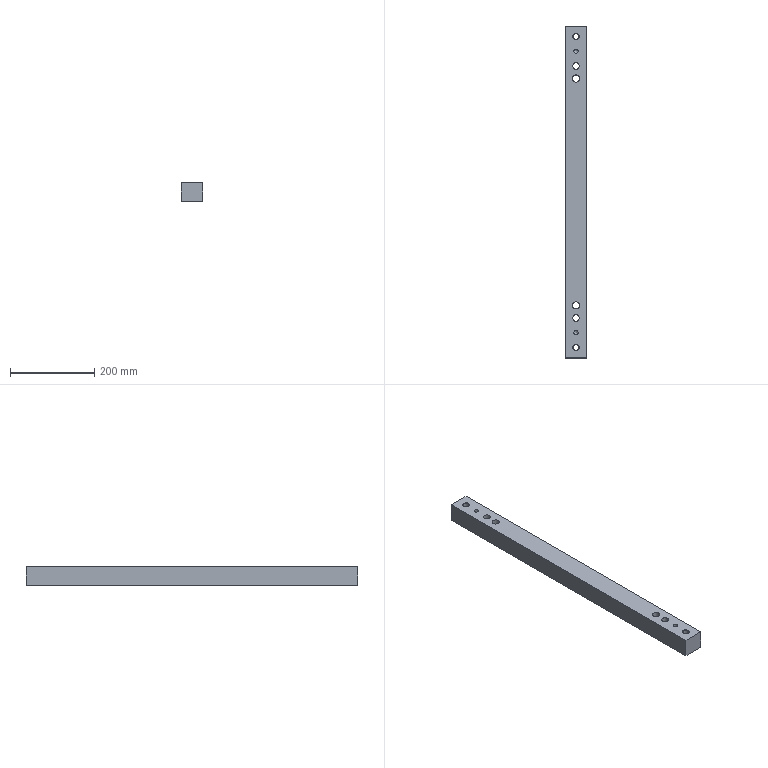Part | STEP file | 011_id2222_x_t | 1 solid | 18 faces | box 50 x 790 x 45 mm | volume 1720407 mm3 | cylinder 8 | plane 6 | cone 4 | commonest cylinder face diameters 10.3 x2 14 x2 16 x2 17 x2
STEP:
#1=CARTESIAN_POINT('',(0.,0.,0.));
#2=DIRECTION('',(0.,0.,1.));
#3=DIRECTION('',(1.,0.,0.));
#4=AXIS2_PLACEMENT_3D('',#1,#2,#3);
#5=CARTESIAN_POINT('',(-933.5,370.,185.));
#6=VERTEX_POINT('',#5);
#7=CARTESIAN_POINT('',(-919.5,370.,185.));
#8=VERTEX_POINT('',#7);
#9=CARTESIAN_POINT('',(-926.5,370.,185.));
#10=DIRECTION('',(0.,0.,-1.));
#11=DIRECTION('',(-1.,0.,0.));
#12=AXIS2_PLACEMENT_3D('',#9,#10,#11);
#13=CIRCLE('',#12,7.);
#14=CARTESIAN_POINT('',(173.5,0.,185.));
#15=DIRECTION('',(0.,0.,-1.));
#16=DIRECTION('',(1.,0.,0.));
#17=AXIS2_PLACEMENT_3D('',#14,#15,#16);
#18=PLANE('',#17);
#19=CARTESIAN_POINT('',(-1100.,-370.));
#20=DIRECTION('',(-1.,0.));
#21=AXIS2_PLACEMENT_2D('',#19,#20);
#22=CIRCLE('',#21,7.);
#23=(GEOMETRIC_REPRESENTATION_CONTEXT(2)PARAMETRIC_REPRESENTATION_CONTEXT()REPRESENTATION_CONTEXT('',''));
#24=DEFINITIONAL_REPRESENTATION('',(#22),#23);
#25=PCURVE('',#18,#24);
#26=CARTESIAN_POINT('',(-926.5,370.,230.));
#27=DIRECTION('',(0.,0.,-1.));
#28=DIRECTION('',(1.,0.,0.));
#29=AXIS2_PLACEMENT_3D('',#26,#27,#28);
#30=CYLINDRICAL_SURFACE('',#29,7.);
#31=CARTESIAN_POINT('',(3.142,45.));
#32=DIRECTION('',(1.,0.));
#33=VECTOR('',#32,1.);
#34=LINE('',#31,#33);
#35=(GEOMETRIC_REPRESENTATION_CONTEXT(2)PARAMETRIC_REPRESENTATION_CONTEXT()REPRESENTATION_CONTEXT('',''));
#36=DEFINITIONAL_REPRESENTATION('',(#34),#35);
#37=PCURVE('',#30,#36);
#38=SURFACE_CURVE('',#13,(#25,#37),.PCURVE_S1.);
#39=EDGE_CURVE('',#6,#8,#38,.T.);
#40=ORIENTED_EDGE('',*,*,#39,.F.);
#41=CARTESIAN_POINT('',(-926.5,370.,185.));
#42=DIRECTION('',(0.,0.,-1.));
#43=DIRECTION('',(-1.,0.,0.));
#44=AXIS2_PLACEMENT_3D('',#41,#42,#43);
#45=CIRCLE('',#44,7.);
#46=CARTESIAN_POINT('',(-1100.,-370.));
#47=DIRECTION('',(-1.,0.));
#48=AXIS2_PLACEMENT_2D('',#46,#47);
#49=CIRCLE('',#48,7.);
#50=(GEOMETRIC_REPRESENTATION_CONTEXT(2)PARAMETRIC_REPRESENTATION_CONTEXT()REPRESENTATION_CONTEXT('',''));
#51=DEFINITIONAL_REPRESENTATION('',(#49),#50);
#52=PCURVE('',#18,#51);
#53=CARTESIAN_POINT('',(-3.142,45.));
#54=DIRECTION('',(1.,0.));
#55=VECTOR('',#54,1.);
#56=LINE('',#53,#55);
#57=(GEOMETRIC_REPRESENTATION_CONTEXT(2)PARAMETRIC_REPRESENTATION_CONTEXT()REPRESENTATION_CONTEXT('',''));
#58=DEFINITIONAL_REPRESENTATION('',(#56),#57);
#59=PCURVE('',#30,#58);
#60=SURFACE_CURVE('',#45,(#52,#59),.PCURVE_S1.);
#61=EDGE_CURVE('',#8,#6,#60,.T.);
#62=ORIENTED_EDGE('',*,*,#61,.F.);
#63=EDGE_LOOP('',(#40,#62));
#64=FACE_BOUND('',#63,.T.);
#65=CARTESIAN_POINT('',(-934.5,-300.,185.));
#66=VERTEX_POINT('',#65);
#67=CARTESIAN_POINT('',(-918.5,-300.,185.));
#68=VERTEX_POINT('',#67);
#69=CARTESIAN_POINT('',(-926.5,-300.,185.));
#70=DIRECTION('',(0.,0.,-1.));
#71=DIRECTION('',(-1.,0.,0.));
#72=AXIS2_PLACEMENT_3D('',#69,#70,#71);
#73=CIRCLE('',#72,8.);
#74=CARTESIAN_POINT('',(-1100.,300.));
#75=DIRECTION('',(-1.,0.));
#76=AXIS2_PLACEMENT_2D('',#74,#75);
#77=CIRCLE('',#76,8.);
#78=(GEOMETRIC_REPRESENTATION_CONTEXT(2)PARAMETRIC_REPRESENTATION_CONTEXT()REPRESENTATION_CONTEXT('',''));
#79=DEFINITIONAL_REPRESENTATION('',(#77),#78);
#80=PCURVE('',#18,#79);
#81=CARTESIAN_POINT('',(-926.5,-300.,310.));
#82=DIRECTION('',(0.,0.,-1.));
#83=DIRECTION('',(1.,0.,0.));
#84=AXIS2_PLACEMENT_3D('',#81,#82,#83);
#85=CYLINDRICAL_SURFACE('',#84,8.);
#86=CARTESIAN_POINT('',(3.142,125.));
#87=DIRECTION('',(1.,0.));
#88=VECTOR('',#87,1.);
#89=LINE('',#86,#88);
#90=(GEOMETRIC_REPRESENTATION_CONTEXT(2)PARAMETRIC_REPRESENTATION_CONTEXT()REPRESENTATION_CONTEXT('',''));
#91=DEFINITIONAL_REPRESENTATION('',(#89),#90);
#92=PCURVE('',#85,#91);
#93=SURFACE_CURVE('',#73,(#80,#92),.PCURVE_S1.);
#94=EDGE_CURVE('',#66,#68,#93,.T.);
#95=ORIENTED_EDGE('',*,*,#94,.F.);
#96=CARTESIAN_POINT('',(-926.5,-300.,185.));
#97=DIRECTION('',(0.,0.,-1.));
#98=DIRECTION('',(-1.,0.,0.));
#99=AXIS2_PLACEMENT_3D('',#96,#97,#98);
#100=CIRCLE('',#99,8.);
#101=CARTESIAN_POINT('',(-1100.,300.));
#102=DIRECTION('',(-1.,0.));
#103=AXIS2_PLACEMENT_2D('',#101,#102);
#104=CIRCLE('',#103,8.);
#105=(GEOMETRIC_REPRESENTATION_CONTEXT(2)PARAMETRIC_REPRESENTATION_CONTEXT()REPRESENTATION_CONTEXT('',''));
#106=DEFINITIONAL_REPRESENTATION('',(#104),#105);
#107=PCURVE('',#18,#106);
#108=CARTESIAN_POINT('',(-3.142,125.));
#109=DIRECTION('',(1.,0.));
#110=VECTOR('',#109,1.);
#111=LINE('',#108,#110);
#112=(GEOMETRIC_REPRESENTATION_CONTEXT(2)PARAMETRIC_REPRESENTATION_CONTEXT()REPRESENTATION_CONTEXT('',''));
#113=DEFINITIONAL_REPRESENTATION('',(#111),#112);
#114=PCURVE('',#85,#113);
#115=SURFACE_CURVE('',#100,(#107,#114),.PCURVE_S1.);
#116=EDGE_CURVE('',#68,#66,#115,.T.);
#117=ORIENTED_EDGE('',*,*,#116,.F.);
#118=EDGE_LOOP('',(#95,#117));
#119=FACE_BOUND('',#118,.T.);
#120=CARTESIAN_POINT('',(-934.5,300.,185.));
#121=VERTEX_POINT('',#120);
#122=CARTESIAN_POINT('',(-918.5,300.,185.));
#123=VERTEX_POINT('',#122);
#124=CARTESIAN_POINT('',(-926.5,300.,185.));
#125=DIRECTION('',(0.,0.,-1.));
#126=DIRECTION('',(-1.,0.,0.));
#127=AXIS2_PLACEMENT_3D('',#124,#125,#126);
#128=CIRCLE('',#127,8.);
#129=CARTESIAN_POINT('',(-1100.,-300.));
#130=DIRECTION('',(-1.,0.));
#131=AXIS2_PLACEMENT_2D('',#129,#130);
#132=CIRCLE('',#131,8.);
#133=(GEOMETRIC_REPRESENTATION_CONTEXT(2)PARAMETRIC_REPRESENTATION_CONTEXT()REPRESENTATION_CONTEXT('',''));
#134=DEFINITIONAL_REPRESENTATION('',(#132),#133);
#135=PCURVE('',#18,#134);
#136=CARTESIAN_POINT('',(-926.5,300.,310.));
#137=DIRECTION('',(0.,0.,-1.));
#138=DIRECTION('',(1.,0.,0.));
#139=AXIS2_PLACEMENT_3D('',#136,#137,#138);
#140=CYLINDRICAL_SURFACE('',#139,8.);
#141=CARTESIAN_POINT('',(3.142,125.));
#142=DIRECTION('',(1.,0.));
#143=VECTOR('',#142,1.);
#144=LINE('',#141,#143);
#145=(GEOMETRIC_REPRESENTATION_CONTEXT(2)PARAMETRIC_REPRESENTATION_CONTEXT()REPRESENTATION_CONTEXT('',''));
#146=DEFINITIONAL_REPRESENTATION('',(#144),#145);
#147=PCURVE('',#140,#146);
#148=SURFACE_CURVE('',#128,(#135,#147),.PCURVE_S1.);
#149=EDGE_CURVE('',#121,#123,#148,.T.);
#150=ORIENTED_EDGE('',*,*,#149,.F.);
#151=CARTESIAN_POINT('',(-926.5,300.,185.));
#152=DIRECTION('',(0.,0.,-1.));
#153=DIRECTION('',(-1.,0.,0.));
#154=AXIS2_PLACEMENT_3D('',#151,#152,#153);
#155=CIRCLE('',#154,8.);
#156=CARTESIAN_POINT('',(-1100.,-300.));
#157=DIRECTION('',(-1.,0.));
#158=AXIS2_PLACEMENT_2D('',#156,#157);
#159=CIRCLE('',#158,8.);
#160=(GEOMETRIC_REPRESENTATION_CONTEXT(2)PARAMETRIC_REPRESENTATION_CONTEXT()REPRESENTATION_CONTEXT('',''));
#161=DEFINITIONAL_REPRESENTATION('',(#159),#160);
#162=PCURVE('',#18,#161);
#163=CARTESIAN_POINT('',(-3.142,125.));
#164=DIRECTION('',(1.,0.));
#165=VECTOR('',#164,1.);
#166=LINE('',#163,#165);
#167=(GEOMETRIC_REPRESENTATION_CONTEXT(2)PARAMETRIC_REPRESENTATION_CONTEXT()REPRESENTATION_CONTEXT('',''));
#168=DEFINITIONAL_REPRESENTATION('',(#166),#167);
#169=PCURVE('',#140,#168);
#170=SURFACE_CURVE('',#155,(#162,#169),.PCURVE_S1.);
#171=EDGE_CURVE('',#123,#121,#170,.T.);
#172=ORIENTED_EDGE('',*,*,#171,.F.);
#173=EDGE_LOOP('',(#150,#172));
#174=FACE_BOUND('',#173,.T.);
#175=CARTESIAN_POINT('',(-951.5,-395.,185.));
#176=VERTEX_POINT('',#175);
#177=CARTESIAN_POINT('',(-951.5,395.,185.));
#178=VERTEX_POINT('',#177);
#179=CARTESIAN_POINT('',(-951.5,0.,185.));
#180=DIRECTION('',(0.,1.,0.));
#181=VECTOR('',#180,1.);
#182=LINE('',#179,#181);
#183=CARTESIAN_POINT('',(-1125.,0.));
#184=DIRECTION('',(0.,-1.));
#185=VECTOR('',#184,1.);
#186=LINE('',#183,#185);
#187=(GEOMETRIC_REPRESENTATION_CONTEXT(2)PARAMETRIC_REPRESENTATION_CONTEXT()REPRESENTATION_CONTEXT('',''));
#188=DEFINITIONAL_REPRESENTATION('',(#186),#187);
#189=PCURVE('',#18,#188);
#190=CARTESIAN_POINT('',(-951.5,-210.,-28.5));
#191=DIRECTION('',(-1.,0.,0.));
#192=DIRECTION('',(0.,0.,1.));
#193=AXIS2_PLACEMENT_3D('',#190,#191,#192);
#194=PLANE('',#193);
#195=CARTESIAN_POINT('',(213.5,210.));
#196=DIRECTION('',(0.,1.));
#197=VECTOR('',#196,1.);
#198=LINE('',#195,#197);
#199=(GEOMETRIC_REPRESENTATION_CONTEXT(2)PARAMETRIC_REPRESENTATION_CONTEXT()REPRESENTATION_CONTEXT('',''));
#200=DEFINITIONAL_REPRESENTATION('',(#198),#199);
#201=PCURVE('',#194,#200);
#202=SURFACE_CURVE('',#182,(#189,#201),.PCURVE_S1.);
#203=EDGE_CURVE('',#176,#178,#202,.T.);
#204=ORIENTED_EDGE('',*,*,#203,.T.);
#205=CARTESIAN_POINT('',(-901.5,395.,185.));
#206=VERTEX_POINT('',#205);
#207=CARTESIAN_POINT('',(-951.5,395.,185.));
#208=DIRECTION('',(-1.,0.,0.));
#209=VECTOR('',#208,1.);
#210=LINE('',#207,#209);
#211=CARTESIAN_POINT('',(-1125.,-395.));
#212=DIRECTION('',(-1.,0.));
#213=VECTOR('',#212,1.);
#214=LINE('',#211,#213);
#215=(GEOMETRIC_REPRESENTATION_CONTEXT(2)PARAMETRIC_REPRESENTATION_CONTEXT()REPRESENTATION_CONTEXT('',''));
#216=DEFINITIONAL_REPRESENTATION('',(#214),#215);
#217=PCURVE('',#18,#216);
#218=CARTESIAN_POINT('',(-951.5,395.,-28.5));
#219=DIRECTION('',(0.,1.,0.));
#220=DIRECTION('',(0.,0.,-1.));
#221=AXIS2_PLACEMENT_3D('',#218,#219,#220);
#222=PLANE('',#221);
#223=CARTESIAN_POINT('',(-213.5,0.));
#224=DIRECTION('',(0.,1.));
#225=VECTOR('',#224,1.);
#226=LINE('',#223,#225);
#227=(GEOMETRIC_REPRESENTATION_CONTEXT(2)PARAMETRIC_REPRESENTATION_CONTEXT()REPRESENTATION_CONTEXT('',''));
#228=DEFINITIONAL_REPRESENTATION('',(#226),#227);
#229=PCURVE('',#222,#228);
#230=SURFACE_CURVE('',#210,(#217,#229),.PCURVE_S1.);
#231=EDGE_CURVE('',#206,#178,#230,.T.);
#232=ORIENTED_EDGE('',*,*,#231,.F.);
#233=CARTESIAN_POINT('',(-901.5,-395.,185.));
#234=VERTEX_POINT('',#233);
#235=CARTESIAN_POINT('',(-901.5,-210.,185.));
#236=DIRECTION('',(0.,-1.,0.));
#237=VECTOR('',#236,1.);
#238=LINE('',#235,#237);
#239=CARTESIAN_POINT('',(-1075.,210.));
#240=DIRECTION('',(0.,1.));
#241=VECTOR('',#240,1.);
#242=LINE('',#239,#241);
#243=(GEOMETRIC_REPRESENTATION_CONTEXT(2)PARAMETRIC_REPRESENTATION_CONTEXT()REPRESENTATION_CONTEXT('',''));
#244=DEFINITIONAL_REPRESENTATION('',(#242),#243);
#245=PCURVE('',#18,#244);
#246=CARTESIAN_POINT('',(-901.5,-210.,-28.5));
#247=DIRECTION('',(-1.,0.,0.));
#248=DIRECTION('',(0.,0.,1.));
#249=AXIS2_PLACEMENT_3D('',#246,#247,#248);
#250=PLANE('',#249);
#251=CARTESIAN_POINT('',(213.5,0.));
#252=DIRECTION('',(0.,-1.));
#253=VECTOR('',#252,1.);
#254=LINE('',#251,#253);
#255=(GEOMETRIC_REPRESENTATION_CONTEXT(2)PARAMETRIC_REPRESENTATION_CONTEXT()REPRESENTATION_CONTEXT('',''));
#256=DEFINITIONAL_REPRESENTATION('',(#254),#255);
#257=PCURVE('',#250,#256);
#258=SURFACE_CURVE('',#238,(#245,#257),.PCURVE_S1.);
#259=EDGE_CURVE('',#206,#234,#258,.T.);
#260=ORIENTED_EDGE('',*,*,#259,.T.);
#261=CARTESIAN_POINT('',(173.5,-395.,185.));
#262=DIRECTION('',(1.,0.,0.));
#263=VECTOR('',#262,1.);
#264=LINE('',#261,#263);
#265=CARTESIAN_POINT('',(0.,395.));
#266=DIRECTION('',(1.,0.));
#267=VECTOR('',#266,1.);
#268=LINE('',#265,#267);
#269=(GEOMETRIC_REPRESENTATION_CONTEXT(2)PARAMETRIC_REPRESENTATION_CONTEXT()REPRESENTATION_CONTEXT('',''));
#270=DEFINITIONAL_REPRESENTATION('',(#268),#269);
#271=PCURVE('',#18,#270);
#272=CARTESIAN_POINT('',(-951.5,-395.,-28.5));
#273=DIRECTION('',(0.,1.,0.));
#274=DIRECTION('',(0.,0.,-1.));
#275=AXIS2_PLACEMENT_3D('',#272,#273,#274);
#276=PLANE('',#275);
#277=CARTESIAN_POINT('',(-213.5,-1125.));
#278=DIRECTION('',(0.,-1.));
#279=VECTOR('',#278,1.);
#280=LINE('',#277,#279);
#281=(GEOMETRIC_REPRESENTATION_CONTEXT(2)PARAMETRIC_REPRESENTATION_CONTEXT()REPRESENTATION_CONTEXT('',''));
#282=DEFINITIONAL_REPRESENTATION('',(#280),#281);
#283=PCURVE('',#276,#282);
#284=SURFACE_CURVE('',#264,(#271,#283),.PCURVE_S1.);
#285=EDGE_CURVE('',#176,#234,#284,.T.);
#286=ORIENTED_EDGE('',*,*,#285,.F.);
#287=EDGE_LOOP('',(#204,#232,#260,#286));
#288=FACE_BOUND('',#287,.T.);
#289=CARTESIAN_POINT('',(-933.5,-370.,185.));
#290=VERTEX_POINT('',#289);
#291=CARTESIAN_POINT('',(-919.5,-370.,185.));
#292=VERTEX_POINT('',#291);
#293=CARTESIAN_POINT('',(-926.5,-370.,185.));
#294=DIRECTION('',(0.,0.,-1.));
#295=DIRECTION('',(-1.,0.,0.));
#296=AXIS2_PLACEMENT_3D('',#293,#294,#295);
#297=CIRCLE('',#296,7.);
#298=CARTESIAN_POINT('',(-1100.,370.));
#299=DIRECTION('',(-1.,0.));
#300=AXIS2_PLACEMENT_2D('',#298,#299);
#301=CIRCLE('',#300,7.);
#302=(GEOMETRIC_REPRESENTATION_CONTEXT(2)PARAMETRIC_REPRESENTATION_CONTEXT()REPRESENTATION_CONTEXT('',''));
#303=DEFINITIONAL_REPRESENTATION('',(#301),#302);
#304=PCURVE('',#18,#303);
#305=CARTESIAN_POINT('',(-926.5,-370.,230.));
#306=DIRECTION('',(0.,0.,-1.));
#307=DIRECTION('',(1.,0.,0.));
#308=AXIS2_PLACEMENT_3D('',#305,#306,#307);
#309=CYLINDRICAL_SURFACE('',#308,7.);
#310=CARTESIAN_POINT('',(3.142,45.));
#311=DIRECTION('',(1.,0.));
#312=VECTOR('',#311,1.);
#313=LINE('',#310,#312);
#314=(GEOMETRIC_REPRESENTATION_CONTEXT(2)PARAMETRIC_REPRESENTATION_CONTEXT()REPRESENTATION_CONTEXT('',''));
#315=DEFINITIONAL_REPRESENTATION('',(#313),#314);
#316=PCURVE('',#309,#315);
#317=SURFACE_CURVE('',#297,(#304,#316),.PCURVE_S1.);
#318=EDGE_CURVE('',#290,#292,#317,.T.);
#319=ORIENTED_EDGE('',*,*,#318,.F.);
#320=CARTESIAN_POINT('',(-926.5,-370.,185.));
#321=DIRECTION('',(0.,0.,-1.));
#322=DIRECTION('',(-1.,0.,0.));
#323=AXIS2_PLACEMENT_3D('',#320,#321,#322);
#324=CIRCLE('',#323,7.);
#325=CARTESIAN_POINT('',(-1100.,370.));
#326=DIRECTION('',(-1.,0.));
#327=AXIS2_PLACEMENT_2D('',#325,#326);
#328=CIRCLE('',#327,7.);
#329=(GEOMETRIC_REPRESENTATION_CONTEXT(2)PARAMETRIC_REPRESENTATION_CONTEXT()REPRESENTATION_CONTEXT('',''));
#330=DEFINITIONAL_REPRESENTATION('',(#328),#329);
#331=PCURVE('',#18,#330);
#332=CARTESIAN_POINT('',(-3.142,45.));
#333=DIRECTION('',(1.,0.));
#334=VECTOR('',#333,1.);
#335=LINE('',#332,#334);
#336=(GEOMETRIC_REPRESENTATION_CONTEXT(2)PARAMETRIC_REPRESENTATION_CONTEXT()REPRESENTATION_CONTEXT('',''));
#337=DEFINITIONAL_REPRESENTATION('',(#335),#336);
#338=PCURVE('',#309,#337);
#339=SURFACE_CURVE('',#324,(#331,#338),.PCURVE_S1.);
#340=EDGE_CURVE('',#292,#290,#339,.T.);
#341=ORIENTED_EDGE('',*,*,#340,.F.);
#342=EDGE_LOOP('',(#319,#341));
#343=FACE_BOUND('',#342,.T.);
#344=CARTESIAN_POINT('',(-935.,-270.,185.));
#345=VERTEX_POINT('',#344);
#346=CARTESIAN_POINT('',(-926.5,-270.,185.));
#347=DIRECTION('',(0.,0.,-1.));
#348=DIRECTION('',(-1.,0.,0.));
#349=AXIS2_PLACEMENT_3D('',#346,#347,#348);
#350=CIRCLE('',#349,8.5);
#351=CARTESIAN_POINT('',(-1100.,270.));
#352=DIRECTION('',(-1.,0.));
#353=AXIS2_PLACEMENT_2D('',#351,#352);
#354=CIRCLE('',#353,8.5);
#355=(GEOMETRIC_REPRESENTATION_CONTEXT(2)PARAMETRIC_REPRESENTATION_CONTEXT()REPRESENTATION_CONTEXT('',''));
#356=DEFINITIONAL_REPRESENTATION('',(#354),#355);
#357=PCURVE('',#18,#356);
#358=CARTESIAN_POINT('',(-926.5,-270.,150.));
#359=DIRECTION('',(0.,0.,1.));
#360=DIRECTION('',(1.,0.,0.));
#361=AXIS2_PLACEMENT_3D('',#358,#359,#360);
#362=CYLINDRICAL_SURFACE('',#361,8.5);
#363=CARTESIAN_POINT('',(9.425,35.));
#364=DIRECTION('',(-1.,0.));
#365=VECTOR('',#364,1.);
#366=LINE('',#363,#365);
#367=(GEOMETRIC_REPRESENTATION_CONTEXT(2)PARAMETRIC_REPRESENTATION_CONTEXT()REPRESENTATION_CONTEXT('',''));
#368=DEFINITIONAL_REPRESENTATION('',(#366),#367);
#369=PCURVE('',#362,#368);
#370=SURFACE_CURVE('',#350,(#357,#369),.PCURVE_S1.);
#371=EDGE_CURVE('',#345,#345,#370,.T.);
#372=ORIENTED_EDGE('',*,*,#371,.F.);
#373=EDGE_LOOP('',(#372));
#374=FACE_BOUND('',#373,.T.);
#375=CARTESIAN_POINT('',(-935.,270.,185.));
#376=VERTEX_POINT('',#375);
#377=CARTESIAN_POINT('',(-926.5,270.,185.));
#378=DIRECTION('',(0.,0.,1.));
#379=DIRECTION('',(-1.,0.,0.));
#380=AXIS2_PLACEMENT_3D('',#377,#378,#379);
#381=CIRCLE('',#380,8.5);
#382=CARTESIAN_POINT('',(-1108.5,-270.));
#383=CARTESIAN_POINT('',(-1108.5,-255.278));
#384=CARTESIAN_POINT('',(-1095.75,-262.639));
#385=CARTESIAN_POINT('',(-1083.,-270.));
#386=CARTESIAN_POINT('',(-1095.75,-277.361));
#387=CARTESIAN_POINT('',(-1108.5,-284.722));
#388=CARTESIAN_POINT('',(-1108.5,-270.));
#389=(BOUNDED_CURVE()B_SPLINE_CURVE(2,(#382,#383,#384,#385,#386,#387,#388),.UNSPECIFIED.,.T.,.F.)B_SPLINE_CURVE_WITH_KNOTS((1,2,2,2,2,1),(-2.094,0.,2.094,4.189,6.283,8.378),.UNSPECIFIED.)CURVE()GEOMETRIC_REPRESENTATION_ITEM()RATIONAL_B_SPLINE_CURVE((1.,0.5,1.,0.5,1.,0.5,1.))REPRESENTATION_ITEM(''));
#390=(GEOMETRIC_REPRESENTATION_CONTEXT(2)PARAMETRIC_REPRESENTATION_CONTEXT()REPRESENTATION_CONTEXT('',''));
#391=DEFINITIONAL_REPRESENTATION('',(#389),#390);
#392=PCURVE('',#18,#391);
#393=CARTESIAN_POINT('',(-926.5,270.,150.));
#394=DIRECTION('',(0.,0.,1.));
#395=DIRECTION('',(1.,0.,0.));
#396=AXIS2_PLACEMENT_3D('',#393,#394,#395);
#397=CYLINDRICAL_SURFACE('',#396,8.5);
#398=CARTESIAN_POINT('',(3.142,35.));
#399=DIRECTION('',(1.,0.));
#400=VECTOR('',#399,1.);
#401=LINE('',#398,#400);
#402=(GEOMETRIC_REPRESENTATION_CONTEXT(2)PARAMETRIC_REPRESENTATION_CONTEXT()REPRESENTATION_CONTEXT('',''));
#403=DEFINITIONAL_REPRESENTATION('',(#401),#402);
#404=PCURVE('',#397,#403);
#405=SURFACE_CURVE('',#381,(#392,#404),.PCURVE_S1.);
#406=EDGE_CURVE('',#376,#376,#405,.T.);
#407=ORIENTED_EDGE('',*,*,#406,.T.);
#408=EDGE_LOOP('',(#407));
#409=FACE_BOUND('',#408,.T.);
#410=ADVANCED_FACE('',(#64,#119,#174,#288,#343,#374,#409),#18,.T.);
#411=CARTESIAN_POINT('',(-931.65,-335.,230.));
#412=VERTEX_POINT('',#411);
#413=CARTESIAN_POINT('',(-926.5,-335.,230.));
#414=DIRECTION('',(0.,0.,-1.));
#415=DIRECTION('',(-1.,0.,0.));
#416=AXIS2_PLACEMENT_3D('',#413,#414,#415);
#417=CIRCLE('',#416,5.15);
#418=CARTESIAN_POINT('',(-951.5,-210.,230.));
#419=DIRECTION('',(0.,0.,-1.));
#420=DIRECTION('',(0.,-1.,0.));
#421=AXIS2_PLACEMENT_3D('',#418,#419,#420);
#422=PLANE('',#421);
#423=CARTESIAN_POINT('',(125.,-25.));
#424=DIRECTION('',(0.,1.));
#425=AXIS2_PLACEMENT_2D('',#423,#424);
#426=CIRCLE('',#425,5.15);
#427=(GEOMETRIC_REPRESENTATION_CONTEXT(2)PARAMETRIC_REPRESENTATION_CONTEXT()REPRESENTATION_CONTEXT('',''));
#428=DEFINITIONAL_REPRESENTATION('',(#426),#427);
#429=PCURVE('',#422,#428);
#430=CARTESIAN_POINT('',(-926.5,-335.,259.));
#431=DIRECTION('',(0.,0.,-1.));
#432=DIRECTION('',(-1.,0.,0.));
#433=AXIS2_PLACEMENT_3D('',#430,#431,#432);
#434=CYLINDRICAL_SURFACE('',#433,5.15);
#435=CARTESIAN_POINT('',(0.,29.));
#436=DIRECTION('',(1.,0.));
#437=VECTOR('',#436,1.);
#438=LINE('',#435,#437);
#439=(GEOMETRIC_REPRESENTATION_CONTEXT(2)PARAMETRIC_REPRESENTATION_CONTEXT()REPRESENTATION_CONTEXT('',''));
#440=DEFINITIONAL_REPRESENTATION('',(#438),#439);
#441=PCURVE('',#434,#440);
#442=SURFACE_CURVE('',#417,(#429,#441),.PCURVE_S1.);
#443=EDGE_CURVE('',#412,#412,#442,.T.);
#444=ORIENTED_EDGE('',*,*,#443,.T.);
#445=EDGE_LOOP('',(#444));
#446=FACE_BOUND('',#445,.T.);
#447=CARTESIAN_POINT('',(-931.65,335.,230.));
#448=VERTEX_POINT('',#447);
#449=CARTESIAN_POINT('',(-926.5,335.,230.));
#450=DIRECTION('',(0.,0.,1.));
#451=DIRECTION('',(-1.,0.,0.));
#452=AXIS2_PLACEMENT_3D('',#449,#450,#451);
#453=CIRCLE('',#452,5.15);
#454=CARTESIAN_POINT('',(-545.,-19.85));
#455=CARTESIAN_POINT('',(-536.08,-19.85));
#456=CARTESIAN_POINT('',(-540.54,-27.575));
#457=CARTESIAN_POINT('',(-545.,-35.3));
#458=CARTESIAN_POINT('',(-549.46,-27.575));
#459=CARTESIAN_POINT('',(-553.92,-19.85));
#460=CARTESIAN_POINT('',(-545.,-19.85));
#461=(BOUNDED_CURVE()B_SPLINE_CURVE(2,(#454,#455,#456,#457,#458,#459,#460),.UNSPECIFIED.,.T.,.F.)B_SPLINE_CURVE_WITH_KNOTS((1,2,2,2,2,1),(-2.094,0.,2.094,4.189,6.283,8.378),.UNSPECIFIED.)CURVE()GEOMETRIC_REPRESENTATION_ITEM()RATIONAL_B_SPLINE_CURVE((1.,0.5,1.,0.5,1.,0.5,1.))REPRESENTATION_ITEM(''));
#462=(GEOMETRIC_REPRESENTATION_CONTEXT(2)PARAMETRIC_REPRESENTATION_CONTEXT()REPRESENTATION_CONTEXT('',''));
#463=DEFINITIONAL_REPRESENTATION('',(#461),#462);
#464=PCURVE('',#422,#463);
#465=CARTESIAN_POINT('',(-926.5,335.,259.));
#466=DIRECTION('',(0.,0.,-1.));
#467=DIRECTION('',(-1.,0.,0.));
#468=AXIS2_PLACEMENT_3D('',#465,#466,#467);
#469=CYLINDRICAL_SURFACE('',#468,5.15);
#470=CARTESIAN_POINT('',(6.283,29.));
#471=DIRECTION('',(-1.,0.));
#472=VECTOR('',#471,1.);
#473=LINE('',#470,#472);
#474=(GEOMETRIC_REPRESENTATION_CONTEXT(2)PARAMETRIC_REPRESENTATION_CONTEXT()REPRESENTATION_CONTEXT('',''));
#475=DEFINITIONAL_REPRESENTATION('',(#473),#474);
#476=PCURVE('',#469,#475);
#477=SURFACE_CURVE('',#453,(#464,#476),.PCURVE_S1.);
#478=EDGE_CURVE('',#448,#448,#477,.T.);
#479=ORIENTED_EDGE('',*,*,#478,.F.);
#480=EDGE_LOOP('',(#479));
#481=FACE_BOUND('',#480,.T.);
#482=CARTESIAN_POINT('',(-935.,270.,230.));
#483=VERTEX_POINT('',#482);
#484=CARTESIAN_POINT('',(-926.5,270.,230.));
#485=DIRECTION('',(0.,0.,1.));
#486=DIRECTION('',(-1.,0.,0.));
#487=AXIS2_PLACEMENT_3D('',#484,#485,#486);
#488=CIRCLE('',#487,8.5);
#489=CARTESIAN_POINT('',(-480.,-16.5));
#490=CARTESIAN_POINT('',(-465.278,-16.5));
#491=CARTESIAN_POINT('',(-472.639,-29.25));
#492=CARTESIAN_POINT('',(-480.,-42.));
#493=CARTESIAN_POINT('',(-487.361,-29.25));
#494=CARTESIAN_POINT('',(-494.722,-16.5));
#495=CARTESIAN_POINT('',(-480.,-16.5));
#496=(BOUNDED_CURVE()B_SPLINE_CURVE(2,(#489,#490,#491,#492,#493,#494,#495),.UNSPECIFIED.,.T.,.F.)B_SPLINE_CURVE_WITH_KNOTS((1,2,2,2,2,1),(-2.094,0.,2.094,4.189,6.283,8.378),.UNSPECIFIED.)CURVE()GEOMETRIC_REPRESENTATION_ITEM()RATIONAL_B_SPLINE_CURVE((1.,0.5,1.,0.5,1.,0.5,1.))REPRESENTATION_ITEM(''));
#497=(GEOMETRIC_REPRESENTATION_CONTEXT(2)PARAMETRIC_REPRESENTATION_CONTEXT()REPRESENTATION_CONTEXT('',''));
#498=DEFINITIONAL_REPRESENTATION('',(#496),#497);
#499=PCURVE('',#422,#498);
#500=CARTESIAN_POINT('',(3.142,80.));
#501=DIRECTION('',(1.,0.));
#502=VECTOR('',#501,1.);
#503=LINE('',#500,#502);
#504=(GEOMETRIC_REPRESENTATION_CONTEXT(2)PARAMETRIC_REPRESENTATION_CONTEXT()REPRESENTATION_CONTEXT('',''));
#505=DEFINITIONAL_REPRESENTATION('',(#503),#504);
#506=PCURVE('',#397,#505);
#507=SURFACE_CURVE('',#488,(#499,#506),.PCURVE_S1.);
#508=EDGE_CURVE('',#483,#483,#507,.T.);
#509=ORIENTED_EDGE('',*,*,#508,.F.);
#510=EDGE_LOOP('',(#509));
#511=FACE_BOUND('',#510,.T.);
#512=CARTESIAN_POINT('',(-935.,-270.,230.));
#513=VERTEX_POINT('',#512);
#514=CARTESIAN_POINT('',(-926.5,-270.,230.));
#515=DIRECTION('',(0.,0.,-1.));
#516=DIRECTION('',(-1.,0.,0.));
#517=AXIS2_PLACEMENT_3D('',#514,#515,#516);
#518=CIRCLE('',#517,8.5);
#519=CARTESIAN_POINT('',(60.,-25.));
#520=DIRECTION('',(0.,1.));
#521=AXIS2_PLACEMENT_2D('',#519,#520);
#522=CIRCLE('',#521,8.5);
#523=(GEOMETRIC_REPRESENTATION_CONTEXT(2)PARAMETRIC_REPRESENTATION_CONTEXT()REPRESENTATION_CONTEXT('',''));
#524=DEFINITIONAL_REPRESENTATION('',(#522),#523);
#525=PCURVE('',#422,#524);
#526=CARTESIAN_POINT('',(9.425,80.));
#527=DIRECTION('',(-1.,0.));
#528=VECTOR('',#527,1.);
#529=LINE('',#526,#528);
#530=(GEOMETRIC_REPRESENTATION_CONTEXT(2)PARAMETRIC_REPRESENTATION_CONTEXT()REPRESENTATION_CONTEXT('',''));
#531=DEFINITIONAL_REPRESENTATION('',(#529),#530);
#532=PCURVE('',#362,#531);
#533=SURFACE_CURVE('',#518,(#525,#532),.PCURVE_S1.);
#534=EDGE_CURVE('',#513,#513,#533,.T.);
#535=ORIENTED_EDGE('',*,*,#534,.T.);
#536=EDGE_LOOP('',(#535));
#537=FACE_BOUND('',#536,.T.);
#538=CARTESIAN_POINT('',(-918.5,300.,230.));
#539=VERTEX_POINT('',#538);
#540=CARTESIAN_POINT('',(-926.5,300.,230.));
#541=DIRECTION('',(0.,0.,-1.));
#542=DIRECTION('',(-1.,0.,0.));
#543=AXIS2_PLACEMENT_3D('',#540,#541,#542);
#544=CIRCLE('',#543,8.);
#545=CARTESIAN_POINT('',(-510.,-25.));
#546=DIRECTION('',(0.,1.));
#547=AXIS2_PLACEMENT_2D('',#545,#546);
#548=CIRCLE('',#547,8.);
#549=(GEOMETRIC_REPRESENTATION_CONTEXT(2)PARAMETRIC_REPRESENTATION_CONTEXT()REPRESENTATION_CONTEXT('',''));
#550=DEFINITIONAL_REPRESENTATION('',(#548),#549);
#551=PCURVE('',#422,#550);
#552=CARTESIAN_POINT('',(-3.142,80.));
#553=DIRECTION('',(1.,0.));
#554=VECTOR('',#553,1.);
#555=LINE('',#552,#554);
#556=(GEOMETRIC_REPRESENTATION_CONTEXT(2)PARAMETRIC_REPRESENTATION_CONTEXT()REPRESENTATION_CONTEXT('',''));
#557=DEFINITIONAL_REPRESENTATION('',(#555),#556);
#558=PCURVE('',#140,#557);
#559=SURFACE_CURVE('',#544,(#551,#558),.PCURVE_S1.);
#560=EDGE_CURVE('',#539,#539,#559,.T.);
#561=ORIENTED_EDGE('',*,*,#560,.T.);
#562=EDGE_LOOP('',(#561));
#563=FACE_BOUND('',#562,.T.);
#564=CARTESIAN_POINT('',(-918.5,370.,230.));
#565=VERTEX_POINT('',#564);
#566=CARTESIAN_POINT('',(-926.5,370.,230.));
#567=DIRECTION('',(0.,0.,1.));
#568=DIRECTION('',(1.,0.,0.));
#569=AXIS2_PLACEMENT_3D('',#566,#567,#568);
#570=CIRCLE('',#569,8.);
#571=CARTESIAN_POINT('',(-580.,-33.));
#572=CARTESIAN_POINT('',(-593.856,-33.));
#573=CARTESIAN_POINT('',(-586.928,-21.));
#574=CARTESIAN_POINT('',(-580.,-9.));
#575=CARTESIAN_POINT('',(-573.072,-21.));
#576=CARTESIAN_POINT('',(-566.144,-33.));
#577=CARTESIAN_POINT('',(-580.,-33.));
#578=(BOUNDED_CURVE()B_SPLINE_CURVE(2,(#571,#572,#573,#574,#575,#576,#577),.UNSPECIFIED.,.T.,.F.)B_SPLINE_CURVE_WITH_KNOTS((1,2,2,2,2,1),(-2.094,0.,2.094,4.189,6.283,8.378),.UNSPECIFIED.)CURVE()GEOMETRIC_REPRESENTATION_ITEM()RATIONAL_B_SPLINE_CURVE((1.,0.5,1.,0.5,1.,0.5,1.))REPRESENTATION_ITEM(''));
#579=(GEOMETRIC_REPRESENTATION_CONTEXT(2)PARAMETRIC_REPRESENTATION_CONTEXT()REPRESENTATION_CONTEXT('',''));
#580=DEFINITIONAL_REPRESENTATION('',(#578),#579);
#581=PCURVE('',#422,#580);
#582=CARTESIAN_POINT('',(-926.5,370.,230.));
#583=DIRECTION('',(0.,0.,1.));
#584=DIRECTION('',(-1.,0.,0.));
#585=AXIS2_PLACEMENT_3D('',#582,#583,#584);
#586=CONICAL_SURFACE('',#585,8.,0.7854);
#587=CARTESIAN_POINT('',(3.142,0.));
#588=DIRECTION('',(1.,0.));
#589=VECTOR('',#588,1.);
#590=LINE('',#587,#589);
#591=(GEOMETRIC_REPRESENTATION_CONTEXT(2)PARAMETRIC_REPRESENTATION_CONTEXT()REPRESENTATION_CONTEXT('',''));
#592=DEFINITIONAL_REPRESENTATION('',(#590),#591);
#593=PCURVE('',#586,#592);
#594=SURFACE_CURVE('',#570,(#581,#593),.PCURVE_S1.);
#595=EDGE_CURVE('',#565,#565,#594,.T.);
#596=ORIENTED_EDGE('',*,*,#595,.F.);
#597=EDGE_LOOP('',(#596));
#598=FACE_BOUND('',#597,.T.);
#599=CARTESIAN_POINT('',(-918.5,-370.,230.));
#600=VERTEX_POINT('',#599);
#601=CARTESIAN_POINT('',(-926.5,-370.,230.));
#602=DIRECTION('',(0.,0.,1.));
#603=DIRECTION('',(1.,0.,0.));
#604=AXIS2_PLACEMENT_3D('',#601,#602,#603);
#605=CIRCLE('',#604,8.);
#606=CARTESIAN_POINT('',(160.,-33.));
#607=CARTESIAN_POINT('',(146.144,-33.));
#608=CARTESIAN_POINT('',(153.072,-21.));
#609=CARTESIAN_POINT('',(160.,-9.));
#610=CARTESIAN_POINT('',(166.928,-21.));
#611=CARTESIAN_POINT('',(173.856,-33.));
#612=CARTESIAN_POINT('',(160.,-33.));
#613=(BOUNDED_CURVE()B_SPLINE_CURVE(2,(#606,#607,#608,#609,#610,#611,#612),.UNSPECIFIED.,.T.,.F.)B_SPLINE_CURVE_WITH_KNOTS((1,2,2,2,2,1),(-2.094,0.,2.094,4.189,6.283,8.378),.UNSPECIFIED.)CURVE()GEOMETRIC_REPRESENTATION_ITEM()RATIONAL_B_SPLINE_CURVE((1.,0.5,1.,0.5,1.,0.5,1.))REPRESENTATION_ITEM(''));
#614=(GEOMETRIC_REPRESENTATION_CONTEXT(2)PARAMETRIC_REPRESENTATION_CONTEXT()REPRESENTATION_CONTEXT('',''));
#615=DEFINITIONAL_REPRESENTATION('',(#613),#614);
#616=PCURVE('',#422,#615);
#617=CARTESIAN_POINT('',(-926.5,-370.,230.));
#618=DIRECTION('',(0.,0.,1.));
#619=DIRECTION('',(-1.,0.,0.));
#620=AXIS2_PLACEMENT_3D('',#617,#618,#619);
#621=CONICAL_SURFACE('',#620,8.,0.7854);
#622=CARTESIAN_POINT('',(3.142,0.));
#623=DIRECTION('',(1.,0.));
#624=VECTOR('',#623,1.);
#625=LINE('',#622,#624);
#626=(GEOMETRIC_REPRESENTATION_CONTEXT(2)PARAMETRIC_REPRESENTATION_CONTEXT()REPRESENTATION_CONTEXT('',''));
#627=DEFINITIONAL_REPRESENTATION('',(#625),#626);
#628=PCURVE('',#621,#627);
#629=SURFACE_CURVE('',#605,(#616,#628),.PCURVE_S1.);
#630=EDGE_CURVE('',#600,#600,#629,.T.);
#631=ORIENTED_EDGE('',*,*,#630,.F.);
#632=EDGE_LOOP('',(#631));
#633=FACE_BOUND('',#632,.T.);
#634=CARTESIAN_POINT('',(-918.5,-300.,230.));
#635=VERTEX_POINT('',#634);
#636=CARTESIAN_POINT('',(-926.5,-300.,230.));
#637=DIRECTION('',(0.,0.,1.));
#638=DIRECTION('',(1.,0.,0.));
#639=AXIS2_PLACEMENT_3D('',#636,#637,#638);
#640=CIRCLE('',#639,8.);
#641=CARTESIAN_POINT('',(90.,-33.));
#642=CARTESIAN_POINT('',(76.144,-33.));
#643=CARTESIAN_POINT('',(83.072,-21.));
#644=CARTESIAN_POINT('',(90.,-9.));
#645=CARTESIAN_POINT('',(96.928,-21.));
#646=CARTESIAN_POINT('',(103.856,-33.));
#647=CARTESIAN_POINT('',(90.,-33.));
#648=(BOUNDED_CURVE()B_SPLINE_CURVE(2,(#641,#642,#643,#644,#645,#646,#647),.UNSPECIFIED.,.T.,.F.)B_SPLINE_CURVE_WITH_KNOTS((1,2,2,2,2,1),(-2.094,0.,2.094,4.189,6.283,8.378),.UNSPECIFIED.)CURVE()GEOMETRIC_REPRESENTATION_ITEM()RATIONAL_B_SPLINE_CURVE((1.,0.5,1.,0.5,1.,0.5,1.))REPRESENTATION_ITEM(''));
#649=(GEOMETRIC_REPRESENTATION_CONTEXT(2)PARAMETRIC_REPRESENTATION_CONTEXT()REPRESENTATION_CONTEXT('',''));
#650=DEFINITIONAL_REPRESENTATION('',(#648),#649);
#651=PCURVE('',#422,#650);
#652=CARTESIAN_POINT('',(6.283,80.));
#653=DIRECTION('',(-1.,0.));
#654=VECTOR('',#653,1.);
#655=LINE('',#652,#654);
#656=(GEOMETRIC_REPRESENTATION_CONTEXT(2)PARAMETRIC_REPRESENTATION_CONTEXT()REPRESENTATION_CONTEXT('',''));
#657=DEFINITIONAL_REPRESENTATION('',(#655),#656);
#658=PCURVE('',#85,#657);
#659=SURFACE_CURVE('',#640,(#651,#658),.PCURVE_S1.);
#660=EDGE_CURVE('',#635,#635,#659,.T.);
#661=ORIENTED_EDGE('',*,*,#660,.F.);
#662=EDGE_LOOP('',(#661));
#663=FACE_BOUND('',#662,.T.);
#664=CARTESIAN_POINT('',(-951.5,-395.,230.));
#665=VERTEX_POINT('',#664);
#666=CARTESIAN_POINT('',(-901.5,-395.,230.));
#667=VERTEX_POINT('',#666);
#668=CARTESIAN_POINT('',(-951.5,-395.,230.));
#669=DIRECTION('',(1.,0.,0.));
#670=VECTOR('',#669,1.);
#671=LINE('',#668,#670);
#672=CARTESIAN_POINT('',(185.,0.));
#673=DIRECTION('',(0.,-1.));
#674=VECTOR('',#673,1.);
#675=LINE('',#672,#674);
#676=(GEOMETRIC_REPRESENTATION_CONTEXT(2)PARAMETRIC_REPRESENTATION_CONTEXT()REPRESENTATION_CONTEXT('',''));
#677=DEFINITIONAL_REPRESENTATION('',(#675),#676);
#678=PCURVE('',#422,#677);
#679=CARTESIAN_POINT('',(-258.5,0.));
#680=DIRECTION('',(0.,-1.));
#681=VECTOR('',#680,1.);
#682=LINE('',#679,#681);
#683=(GEOMETRIC_REPRESENTATION_CONTEXT(2)PARAMETRIC_REPRESENTATION_CONTEXT()REPRESENTATION_CONTEXT('',''));
#684=DEFINITIONAL_REPRESENTATION('',(#682),#683);
#685=PCURVE('',#276,#684);
#686=SURFACE_CURVE('',#671,(#678,#685),.PCURVE_S1.);
#687=EDGE_CURVE('',#665,#667,#686,.T.);
#688=ORIENTED_EDGE('',*,*,#687,.T.);
#689=CARTESIAN_POINT('',(-901.5,395.,230.));
#690=VERTEX_POINT('',#689);
#691=CARTESIAN_POINT('',(-901.5,-210.,230.));
#692=DIRECTION('',(0.,-1.,0.));
#693=VECTOR('',#692,1.);
#694=LINE('',#691,#693);
#695=CARTESIAN_POINT('',(0.,-50.));
#696=DIRECTION('',(1.,0.));
#697=VECTOR('',#696,1.);
#698=LINE('',#695,#697);
#699=(GEOMETRIC_REPRESENTATION_CONTEXT(2)PARAMETRIC_REPRESENTATION_CONTEXT()REPRESENTATION_CONTEXT('',''));
#700=DEFINITIONAL_REPRESENTATION('',(#698),#699);
#701=PCURVE('',#422,#700);
#702=CARTESIAN_POINT('',(258.5,0.));
#703=DIRECTION('',(0.,-1.));
#704=VECTOR('',#703,1.);
#705=LINE('',#702,#704);
#706=(GEOMETRIC_REPRESENTATION_CONTEXT(2)PARAMETRIC_REPRESENTATION_CONTEXT()REPRESENTATION_CONTEXT('',''));
#707=DEFINITIONAL_REPRESENTATION('',(#705),#706);
#708=PCURVE('',#250,#707);
#709=SURFACE_CURVE('',#694,(#701,#708),.PCURVE_S1.);
#710=EDGE_CURVE('',#690,#667,#709,.T.);
#711=ORIENTED_EDGE('',*,*,#710,.F.);
#712=CARTESIAN_POINT('',(-951.5,395.,230.));
#713=VERTEX_POINT('',#712);
#714=CARTESIAN_POINT('',(-951.5,395.,230.));
#715=DIRECTION('',(1.,0.,0.));
#716=VECTOR('',#715,1.);
#717=LINE('',#714,#716);
#718=CARTESIAN_POINT('',(-605.,0.));
#719=DIRECTION('',(0.,-1.));
#720=VECTOR('',#719,1.);
#721=LINE('',#718,#720);
#722=(GEOMETRIC_REPRESENTATION_CONTEXT(2)PARAMETRIC_REPRESENTATION_CONTEXT()REPRESENTATION_CONTEXT('',''));
#723=DEFINITIONAL_REPRESENTATION('',(#721),#722);
#724=PCURVE('',#422,#723);
#725=CARTESIAN_POINT('',(-258.5,0.));
#726=DIRECTION('',(0.,-1.));
#727=VECTOR('',#726,1.);
#728=LINE('',#725,#727);
#729=(GEOMETRIC_REPRESENTATION_CONTEXT(2)PARAMETRIC_REPRESENTATION_CONTEXT()REPRESENTATION_CONTEXT('',''));
#730=DEFINITIONAL_REPRESENTATION('',(#728),#729);
#731=PCURVE('',#222,#730);
#732=SURFACE_CURVE('',#717,(#724,#731),.PCURVE_S1.);
#733=EDGE_CURVE('',#713,#690,#732,.T.);
#734=ORIENTED_EDGE('',*,*,#733,.F.);
#735=CARTESIAN_POINT('',(-951.5,-210.,230.));
#736=DIRECTION('',(0.,-1.,0.));
#737=VECTOR('',#736,1.);
#738=LINE('',#735,#737);
#739=CARTESIAN_POINT('',(0.,0.));
#740=DIRECTION('',(1.,0.));
#741=VECTOR('',#740,1.);
#742=LINE('',#739,#741);
#743=(GEOMETRIC_REPRESENTATION_CONTEXT(2)PARAMETRIC_REPRESENTATION_CONTEXT()REPRESENTATION_CONTEXT('',''));
#744=DEFINITIONAL_REPRESENTATION('',(#742),#743);
#745=PCURVE('',#422,#744);
#746=CARTESIAN_POINT('',(258.5,0.));
#747=DIRECTION('',(0.,-1.));
#748=VECTOR('',#747,1.);
#749=LINE('',#746,#748);
#750=(GEOMETRIC_REPRESENTATION_CONTEXT(2)PARAMETRIC_REPRESENTATION_CONTEXT()REPRESENTATION_CONTEXT('',''));
#751=DEFINITIONAL_REPRESENTATION('',(#749),#750);
#752=PCURVE('',#194,#751);
#753=SURFACE_CURVE('',#738,(#745,#752),.PCURVE_S1.);
#754=EDGE_CURVE('',#713,#665,#753,.T.);
#755=ORIENTED_EDGE('',*,*,#754,.T.);
#756=EDGE_LOOP('',(#688,#711,#734,#755));
#757=FACE_BOUND('',#756,.T.);
#758=ADVANCED_FACE('',(#446,#481,#511,#537,#563,#598,#633,#663,#757),#422,.F.);
#759=ORIENTED_EDGE('',*,*,#285,.T.);
#760=CARTESIAN_POINT('',(-901.5,-395.,-28.5));
#761=DIRECTION('',(0.,0.,-1.));
#762=VECTOR('',#761,1.);
#763=LINE('',#760,#762);
#764=CARTESIAN_POINT('',(0.,-50.));
#765=DIRECTION('',(1.,0.));
#766=VECTOR('',#765,1.);
#767=LINE('',#764,#766);
#768=(GEOMETRIC_REPRESENTATION_CONTEXT(2)PARAMETRIC_REPRESENTATION_CONTEXT()REPRESENTATION_CONTEXT('',''));
#769=DEFINITIONAL_REPRESENTATION('',(#767),#768);
#770=PCURVE('',#276,#769);
#771=CARTESIAN_POINT('',(0.,-185.));
#772=DIRECTION('',(-1.,0.));
#773=VECTOR('',#772,1.);
#774=LINE('',#771,#773);
#775=(GEOMETRIC_REPRESENTATION_CONTEXT(2)PARAMETRIC_REPRESENTATION_CONTEXT()REPRESENTATION_CONTEXT('',''));
#776=DEFINITIONAL_REPRESENTATION('',(#774),#775);
#777=PCURVE('',#250,#776);
#778=SURFACE_CURVE('',#763,(#770,#777),.PCURVE_S1.);
#779=EDGE_CURVE('',#667,#234,#778,.T.);
#780=ORIENTED_EDGE('',*,*,#779,.F.);
#781=ORIENTED_EDGE('',*,*,#687,.F.);
#782=CARTESIAN_POINT('',(-951.5,-395.,-28.5));
#783=DIRECTION('',(0.,0.,-1.));
#784=VECTOR('',#783,1.);
#785=LINE('',#782,#784);
#786=CARTESIAN_POINT('',(0.,0.));
#787=DIRECTION('',(1.,0.));
#788=VECTOR('',#787,1.);
#789=LINE('',#786,#788);
#790=(GEOMETRIC_REPRESENTATION_CONTEXT(2)PARAMETRIC_REPRESENTATION_CONTEXT()REPRESENTATION_CONTEXT('',''));
#791=DEFINITIONAL_REPRESENTATION('',(#789),#790);
#792=PCURVE('',#276,#791);
#793=CARTESIAN_POINT('',(0.,-185.));
#794=DIRECTION('',(-1.,0.));
#795=VECTOR('',#794,1.);
#796=LINE('',#793,#795);
#797=(GEOMETRIC_REPRESENTATION_CONTEXT(2)PARAMETRIC_REPRESENTATION_CONTEXT()REPRESENTATION_CONTEXT('',''));
#798=DEFINITIONAL_REPRESENTATION('',(#796),#797);
#799=PCURVE('',#194,#798);
#800=SURFACE_CURVE('',#785,(#792,#799),.PCURVE_S1.);
#801=EDGE_CURVE('',#665,#176,#800,.T.);
#802=ORIENTED_EDGE('',*,*,#801,.T.);
#803=EDGE_LOOP('',(#759,#780,#781,#802));
#804=FACE_BOUND('',#803,.T.);
#805=ADVANCED_FACE('',(#804),#276,.F.);
#806=ORIENTED_EDGE('',*,*,#259,.F.);
#807=CARTESIAN_POINT('',(-901.5,395.,-28.5));
#808=DIRECTION('',(0.,0.,1.));
#809=VECTOR('',#808,1.);
#810=LINE('',#807,#809);
#811=CARTESIAN_POINT('',(0.,605.));
#812=DIRECTION('',(1.,0.));
#813=VECTOR('',#812,1.);
#814=LINE('',#811,#813);
#815=(GEOMETRIC_REPRESENTATION_CONTEXT(2)PARAMETRIC_REPRESENTATION_CONTEXT()REPRESENTATION_CONTEXT('',''));
#816=DEFINITIONAL_REPRESENTATION('',(#814),#815);
#817=PCURVE('',#250,#816);
#818=CARTESIAN_POINT('',(0.,-50.));
#819=DIRECTION('',(-1.,0.));
#820=VECTOR('',#819,1.);
#821=LINE('',#818,#820);
#822=(GEOMETRIC_REPRESENTATION_CONTEXT(2)PARAMETRIC_REPRESENTATION_CONTEXT()REPRESENTATION_CONTEXT('',''));
#823=DEFINITIONAL_REPRESENTATION('',(#821),#822);
#824=PCURVE('',#222,#823);
#825=SURFACE_CURVE('',#810,(#817,#824),.PCURVE_S1.);
#826=EDGE_CURVE('',#206,#690,#825,.T.);
#827=ORIENTED_EDGE('',*,*,#826,.T.);
#828=ORIENTED_EDGE('',*,*,#710,.T.);
#829=ORIENTED_EDGE('',*,*,#779,.T.);
#830=EDGE_LOOP('',(#806,#827,#828,#829));
#831=FACE_BOUND('',#830,.T.);
#832=ADVANCED_FACE('',(#831),#250,.F.);
#833=ORIENTED_EDGE('',*,*,#826,.F.);
#834=ORIENTED_EDGE('',*,*,#231,.T.);
#835=CARTESIAN_POINT('',(-951.5,395.,-28.5));
#836=DIRECTION('',(0.,0.,1.));
#837=VECTOR('',#836,1.);
#838=LINE('',#835,#837);
#839=CARTESIAN_POINT('',(0.,0.));
#840=DIRECTION('',(-1.,0.));
#841=VECTOR('',#840,1.);
#842=LINE('',#839,#841);
#843=(GEOMETRIC_REPRESENTATION_CONTEXT(2)PARAMETRIC_REPRESENTATION_CONTEXT()REPRESENTATION_CONTEXT('',''));
#844=DEFINITIONAL_REPRESENTATION('',(#842),#843);
#845=PCURVE('',#222,#844);
#846=CARTESIAN_POINT('',(0.,605.));
#847=DIRECTION('',(1.,0.));
#848=VECTOR('',#847,1.);
#849=LINE('',#846,#848);
#850=(GEOMETRIC_REPRESENTATION_CONTEXT(2)PARAMETRIC_REPRESENTATION_CONTEXT()REPRESENTATION_CONTEXT('',''));
#851=DEFINITIONAL_REPRESENTATION('',(#849),#850);
#852=PCURVE('',#194,#851);
#853=SURFACE_CURVE('',#838,(#845,#852),.PCURVE_S1.);
#854=EDGE_CURVE('',#178,#713,#853,.T.);
#855=ORIENTED_EDGE('',*,*,#854,.T.);
#856=ORIENTED_EDGE('',*,*,#733,.T.);
#857=EDGE_LOOP('',(#833,#834,#855,#856));
#858=FACE_BOUND('',#857,.T.);
#859=ADVANCED_FACE('',(#858),#222,.T.);
#860=ORIENTED_EDGE('',*,*,#854,.F.);
#861=ORIENTED_EDGE('',*,*,#203,.F.);
#862=ORIENTED_EDGE('',*,*,#801,.F.);
#863=ORIENTED_EDGE('',*,*,#754,.F.);
#864=EDGE_LOOP('',(#860,#861,#862,#863));
#865=FACE_BOUND('',#864,.T.);
#866=ADVANCED_FACE('',(#865),#194,.T.);
#867=ORIENTED_EDGE('',*,*,#660,.F.);
#868=CARTESIAN_POINT('',(-918.5,-300.,230.));
#869=CARTESIAN_POINT('',(-918.5,-300.,185.));
#870=B_SPLINE_CURVE_WITH_KNOTS('',1,(#868,#869),.UNSPECIFIED.,.F.,.F.,(2,2),(80.,125.),.PIECEWISE_BEZIER_KNOTS.);
#871=CARTESIAN_POINT('',(6.283,0.));
#872=DIRECTION('',(0.,1.));
#873=VECTOR('',#872,1.);
#874=LINE('',#871,#873);
#875=(GEOMETRIC_REPRESENTATION_CONTEXT(2)PARAMETRIC_REPRESENTATION_CONTEXT()REPRESENTATION_CONTEXT('',''));
#876=DEFINITIONAL_REPRESENTATION('',(#874),#875);
#877=PCURVE('',#85,#876);
#878=CARTESIAN_POINT('',(0.,0.));
#879=DIRECTION('',(0.,1.));
#880=VECTOR('',#879,1.);
#881=LINE('',#878,#880);
#882=(GEOMETRIC_REPRESENTATION_CONTEXT(2)PARAMETRIC_REPRESENTATION_CONTEXT()REPRESENTATION_CONTEXT('',''));
#883=DEFINITIONAL_REPRESENTATION('',(#881),#882);
#884=PCURVE('',#85,#883);
#885=SEAM_CURVE('',#870,(#877,#884),.PCURVE_S1.);
#886=EDGE_CURVE('',#635,#68,#885,.T.);
#887=ORIENTED_EDGE('',*,*,#886,.T.);
#888=ORIENTED_EDGE('',*,*,#94,.F.);
#889=ORIENTED_EDGE('',*,*,#116,.F.);
#890=ORIENTED_EDGE('',*,*,#886,.F.);
#891=EDGE_LOOP('',(#867,#887,#888,#889,#890));
#892=FACE_BOUND('',#891,.F.);
#893=ADVANCED_FACE('',(#892),#85,.F.);
#894=ORIENTED_EDGE('',*,*,#560,.T.);
#895=CARTESIAN_POINT('',(-918.5,300.,230.));
#896=CARTESIAN_POINT('',(-918.5,300.,185.));
#897=B_SPLINE_CURVE_WITH_KNOTS('',1,(#895,#896),.UNSPECIFIED.,.F.,.F.,(2,2),(80.,125.),.PIECEWISE_BEZIER_KNOTS.);
#898=CARTESIAN_POINT('',(6.283,0.));
#899=DIRECTION('',(0.,1.));
#900=VECTOR('',#899,1.);
#901=LINE('',#898,#900);
#902=(GEOMETRIC_REPRESENTATION_CONTEXT(2)PARAMETRIC_REPRESENTATION_CONTEXT()REPRESENTATION_CONTEXT('',''));
#903=DEFINITIONAL_REPRESENTATION('',(#901),#902);
#904=PCURVE('',#140,#903);
#905=CARTESIAN_POINT('',(0.,0.));
#906=DIRECTION('',(0.,1.));
#907=VECTOR('',#906,1.);
#908=LINE('',#905,#907);
#909=(GEOMETRIC_REPRESENTATION_CONTEXT(2)PARAMETRIC_REPRESENTATION_CONTEXT()REPRESENTATION_CONTEXT('',''));
#910=DEFINITIONAL_REPRESENTATION('',(#908),#909);
#911=PCURVE('',#140,#910);
#912=SEAM_CURVE('',#897,(#904,#911),.PCURVE_S1.);
#913=EDGE_CURVE('',#539,#123,#912,.T.);
#914=ORIENTED_EDGE('',*,*,#913,.T.);
#915=ORIENTED_EDGE('',*,*,#149,.F.);
#916=ORIENTED_EDGE('',*,*,#171,.F.);
#917=ORIENTED_EDGE('',*,*,#913,.F.);
#918=EDGE_LOOP('',(#894,#914,#915,#916,#917));
#919=FACE_BOUND('',#918,.F.);
#920=ADVANCED_FACE('',(#919),#140,.F.);
#921=CARTESIAN_POINT('',(-919.5,370.,229.));
#922=VERTEX_POINT('',#921);
#923=CARTESIAN_POINT('',(-926.5,370.,229.));
#924=DIRECTION('',(0.,0.,-1.));
#925=DIRECTION('',(1.,0.,0.));
#926=AXIS2_PLACEMENT_3D('',#923,#924,#925);
#927=CIRCLE('',#926,7.);
#928=CARTESIAN_POINT('',(9.425,-1.));
#929=DIRECTION('',(-1.,0.));
#930=VECTOR('',#929,1.);
#931=LINE('',#928,#930);
#932=(GEOMETRIC_REPRESENTATION_CONTEXT(2)PARAMETRIC_REPRESENTATION_CONTEXT()REPRESENTATION_CONTEXT('',''));
#933=DEFINITIONAL_REPRESENTATION('',(#931),#932);
#934=PCURVE('',#586,#933);
#935=CARTESIAN_POINT('',(0.,1.));
#936=DIRECTION('',(1.,0.));
#937=VECTOR('',#936,1.);
#938=LINE('',#935,#937);
#939=(GEOMETRIC_REPRESENTATION_CONTEXT(2)PARAMETRIC_REPRESENTATION_CONTEXT()REPRESENTATION_CONTEXT('',''));
#940=DEFINITIONAL_REPRESENTATION('',(#938),#939);
#941=PCURVE('',#30,#940);
#942=SURFACE_CURVE('',#927,(#934,#941),.PCURVE_S1.);
#943=EDGE_CURVE('',#922,#922,#942,.T.);
#944=ORIENTED_EDGE('',*,*,#943,.F.);
#945=CARTESIAN_POINT('',(-919.5,370.,229.));
#946=CARTESIAN_POINT('',(-918.5,370.,230.));
#947=B_SPLINE_CURVE_WITH_KNOTS('',1,(#945,#946),.UNSPECIFIED.,.F.,.F.,(2,2),(-1.414,0.),.PIECEWISE_BEZIER_KNOTS.);
#948=CARTESIAN_POINT('',(9.425,0.));
#949=DIRECTION('',(0.,1.));
#950=VECTOR('',#949,1.);
#951=LINE('',#948,#950);
#952=(GEOMETRIC_REPRESENTATION_CONTEXT(2)PARAMETRIC_REPRESENTATION_CONTEXT()REPRESENTATION_CONTEXT('',''));
#953=DEFINITIONAL_REPRESENTATION('',(#951),#952);
#954=PCURVE('',#586,#953);
#955=CARTESIAN_POINT('',(3.142,0.));
#956=DIRECTION('',(0.,1.));
#957=VECTOR('',#956,1.);
#958=LINE('',#955,#957);
#959=(GEOMETRIC_REPRESENTATION_CONTEXT(2)PARAMETRIC_REPRESENTATION_CONTEXT()REPRESENTATION_CONTEXT('',''));
#960=DEFINITIONAL_REPRESENTATION('',(#958),#959);
#961=PCURVE('',#586,#960);
#962=SEAM_CURVE('',#947,(#954,#961),.PCURVE_S1.);
#963=EDGE_CURVE('',#922,#565,#962,.T.);
#964=ORIENTED_EDGE('',*,*,#963,.T.);
#965=ORIENTED_EDGE('',*,*,#595,.F.);
#966=ORIENTED_EDGE('',*,*,#963,.F.);
#967=EDGE_LOOP('',(#944,#964,#965,#966));
#968=FACE_BOUND('',#967,.F.);
#969=ADVANCED_FACE('',(#968),#586,.F.);
#970=ORIENTED_EDGE('',*,*,#943,.T.);
#971=CARTESIAN_POINT('',(-919.5,370.,229.));
#972=CARTESIAN_POINT('',(-919.5,370.,185.));
#973=B_SPLINE_CURVE_WITH_KNOTS('',1,(#971,#972),.UNSPECIFIED.,.F.,.F.,(2,2),(1.,45.),.PIECEWISE_BEZIER_KNOTS.);
#974=CARTESIAN_POINT('',(6.283,0.));
#975=DIRECTION('',(0.,1.));
#976=VECTOR('',#975,1.);
#977=LINE('',#974,#976);
#978=(GEOMETRIC_REPRESENTATION_CONTEXT(2)PARAMETRIC_REPRESENTATION_CONTEXT()REPRESENTATION_CONTEXT('',''));
#979=DEFINITIONAL_REPRESENTATION('',(#977),#978);
#980=PCURVE('',#30,#979);
#981=CARTESIAN_POINT('',(0.,0.));
#982=DIRECTION('',(0.,1.));
#983=VECTOR('',#982,1.);
#984=LINE('',#981,#983);
#985=(GEOMETRIC_REPRESENTATION_CONTEXT(2)PARAMETRIC_REPRESENTATION_CONTEXT()REPRESENTATION_CONTEXT('',''));
#986=DEFINITIONAL_REPRESENTATION('',(#984),#985);
#987=PCURVE('',#30,#986);
#988=SEAM_CURVE('',#973,(#980,#987),.PCURVE_S1.);
#989=EDGE_CURVE('',#922,#8,#988,.T.);
#990=ORIENTED_EDGE('',*,*,#989,.T.);
#991=ORIENTED_EDGE('',*,*,#39,.F.);
#992=ORIENTED_EDGE('',*,*,#61,.F.);
#993=ORIENTED_EDGE('',*,*,#989,.F.);
#994=EDGE_LOOP('',(#970,#990,#991,#992,#993));
#995=FACE_BOUND('',#994,.F.);
#996=ADVANCED_FACE('',(#995),#30,.F.);
#997=CARTESIAN_POINT('',(-919.5,-370.,229.));
#998=VERTEX_POINT('',#997);
#999=CARTESIAN_POINT('',(-926.5,-370.,229.));
#1000=DIRECTION('',(0.,0.,-1.));
#1001=DIRECTION('',(1.,0.,0.));
#1002=AXIS2_PLACEMENT_3D('',#999,#1000,#1001);
#1003=CIRCLE('',#1002,7.);
#1004=CARTESIAN_POINT('',(9.425,-1.));
#1005=DIRECTION('',(-1.,0.));
#1006=VECTOR('',#1005,1.);
#1007=LINE('',#1004,#1006);
#1008=(GEOMETRIC_REPRESENTATION_CONTEXT(2)PARAMETRIC_REPRESENTATION_CONTEXT()REPRESENTATION_CONTEXT('',''));
#1009=DEFINITIONAL_REPRESENTATION('',(#1007),#1008);
#1010=PCURVE('',#621,#1009);
#1011=CARTESIAN_POINT('',(0.,1.));
#1012=DIRECTION('',(1.,0.));
#1013=VECTOR('',#1012,1.);
#1014=LINE('',#1011,#1013);
#1015=(GEOMETRIC_REPRESENTATION_CONTEXT(2)PARAMETRIC_REPRESENTATION_CONTEXT()REPRESENTATION_CONTEXT('',''));
#1016=DEFINITIONAL_REPRESENTATION('',(#1014),#1015);
#1017=PCURVE('',#309,#1016);
#1018=SURFACE_CURVE('',#1003,(#1010,#1017),.PCURVE_S1.);
#1019=EDGE_CURVE('',#998,#998,#1018,.T.);
#1020=ORIENTED_EDGE('',*,*,#1019,.F.);
#1021=CARTESIAN_POINT('',(-919.5,-370.,229.));
#1022=CARTESIAN_POINT('',(-918.5,-370.,230.));
#1023=B_SPLINE_CURVE_WITH_KNOTS('',1,(#1021,#1022),.UNSPECIFIED.,.F.,.F.,(2,2),(-1.414,0.),.PIECEWISE_BEZIER_KNOTS.);
#1024=CARTESIAN_POINT('',(9.425,0.));
#1025=DIRECTION('',(0.,1.));
#1026=VECTOR('',#1025,1.);
#1027=LINE('',#1024,#1026);
#1028=(GEOMETRIC_REPRESENTATION_CONTEXT(2)PARAMETRIC_REPRESENTATION_CONTEXT()REPRESENTATION_CONTEXT('',''));
#1029=DEFINITIONAL_REPRESENTATION('',(#1027),#1028);
#1030=PCURVE('',#621,#1029);
#1031=CARTESIAN_POINT('',(3.142,0.));
#1032=DIRECTION('',(0.,1.));
#1033=VECTOR('',#1032,1.);
#1034=LINE('',#1031,#1033);
#1035=(GEOMETRIC_REPRESENTATION_CONTEXT(2)PARAMETRIC_REPRESENTATION_CONTEXT()REPRESENTATION_CONTEXT('',''));
#1036=DEFINITIONAL_REPRESENTATION('',(#1034),#1035);
#1037=PCURVE('',#621,#1036);
#1038=SEAM_CURVE('',#1023,(#1030,#1037),.PCURVE_S1.);
#1039=EDGE_CURVE('',#998,#600,#1038,.T.);
#1040=ORIENTED_EDGE('',*,*,#1039,.T.);
#1041=ORIENTED_EDGE('',*,*,#630,.F.);
#1042=ORIENTED_EDGE('',*,*,#1039,.F.);
#1043=EDGE_LOOP('',(#1020,#1040,#1041,#1042));
#1044=FACE_BOUND('',#1043,.F.);
#1045=ADVANCED_FACE('',(#1044),#621,.F.);
#1046=ORIENTED_EDGE('',*,*,#1019,.T.);
#1047=CARTESIAN_POINT('',(-919.5,-370.,229.));
#1048=CARTESIAN_POINT('',(-919.5,-370.,185.));
#1049=B_SPLINE_CURVE_WITH_KNOTS('',1,(#1047,#1048),.UNSPECIFIED.,.F.,.F.,(2,2),(1.,45.),.PIECEWISE_BEZIER_KNOTS.);
#1050=CARTESIAN_POINT('',(6.283,0.));
#1051=DIRECTION('',(0.,1.));
#1052=VECTOR('',#1051,1.);
#1053=LINE('',#1050,#1052);
#1054=(GEOMETRIC_REPRESENTATION_CONTEXT(2)PARAMETRIC_REPRESENTATION_CONTEXT()REPRESENTATION_CONTEXT('',''));
#1055=DEFINITIONAL_REPRESENTATION('',(#1053),#1054);
#1056=PCURVE('',#309,#1055);
#1057=CARTESIAN_POINT('',(0.,0.));
#1058=DIRECTION('',(0.,1.));
#1059=VECTOR('',#1058,1.);
#1060=LINE('',#1057,#1059);
#1061=(GEOMETRIC_REPRESENTATION_CONTEXT(2)PARAMETRIC_REPRESENTATION_CONTEXT()REPRESENTATION_CONTEXT('',''));
#1062=DEFINITIONAL_REPRESENTATION('',(#1060),#1061);
#1063=PCURVE('',#309,#1062);
#1064=SEAM_CURVE('',#1049,(#1056,#1063),.PCURVE_S1.);
#1065=EDGE_CURVE('',#998,#292,#1064,.T.);
#1066=ORIENTED_EDGE('',*,*,#1065,.T.);
#1067=ORIENTED_EDGE('',*,*,#318,.F.);
#1068=ORIENTED_EDGE('',*,*,#340,.F.);
#1069=ORIENTED_EDGE('',*,*,#1065,.F.);
#1070=EDGE_LOOP('',(#1046,#1066,#1067,#1068,#1069));
#1071=FACE_BOUND('',#1070,.F.);
#1072=ADVANCED_FACE('',(#1071),#309,.F.);
#1073=ORIENTED_EDGE('',*,*,#371,.F.);
#1074=CARTESIAN_POINT('',(-935.,-270.,185.));
#1075=CARTESIAN_POINT('',(-935.,-270.,230.));
#1076=B_SPLINE_CURVE_WITH_KNOTS('',1,(#1074,#1075),.UNSPECIFIED.,.F.,.F.,(2,2),(35.,80.),.PIECEWISE_BEZIER_KNOTS.);
#1077=CARTESIAN_POINT('',(9.425,0.));
#1078=DIRECTION('',(0.,1.));
#1079=VECTOR('',#1078,1.);
#1080=LINE('',#1077,#1079);
#1081=(GEOMETRIC_REPRESENTATION_CONTEXT(2)PARAMETRIC_REPRESENTATION_CONTEXT()REPRESENTATION_CONTEXT('',''));
#1082=DEFINITIONAL_REPRESENTATION('',(#1080),#1081);
#1083=PCURVE('',#362,#1082);
#1084=CARTESIAN_POINT('',(3.142,0.));
#1085=DIRECTION('',(0.,1.));
#1086=VECTOR('',#1085,1.);
#1087=LINE('',#1084,#1086);
#1088=(GEOMETRIC_REPRESENTATION_CONTEXT(2)PARAMETRIC_REPRESENTATION_CONTEXT()REPRESENTATION_CONTEXT('',''));
#1089=DEFINITIONAL_REPRESENTATION('',(#1087),#1088);
#1090=PCURVE('',#362,#1089);
#1091=SEAM_CURVE('',#1076,(#1083,#1090),.PCURVE_S1.);
#1092=EDGE_CURVE('',#345,#513,#1091,.T.);
#1093=ORIENTED_EDGE('',*,*,#1092,.T.);
#1094=ORIENTED_EDGE('',*,*,#534,.T.);
#1095=ORIENTED_EDGE('',*,*,#1092,.F.);
#1096=EDGE_LOOP('',(#1073,#1093,#1094,#1095));
#1097=FACE_BOUND('',#1096,.F.);
#1098=ADVANCED_FACE('',(#1097),#362,.F.);
#1099=ORIENTED_EDGE('',*,*,#406,.T.);
#1100=CARTESIAN_POINT('',(-935.,270.,185.));
#1101=CARTESIAN_POINT('',(-935.,270.,230.));
#1102=B_SPLINE_CURVE_WITH_KNOTS('',1,(#1100,#1101),.UNSPECIFIED.,.F.,.F.,(2,2),(35.,80.),.PIECEWISE_BEZIER_KNOTS.);
#1103=CARTESIAN_POINT('',(9.425,0.));
#1104=DIRECTION('',(0.,1.));
#1105=VECTOR('',#1104,1.);
#1106=LINE('',#1103,#1105);
#1107=(GEOMETRIC_REPRESENTATION_CONTEXT(2)PARAMETRIC_REPRESENTATION_CONTEXT()REPRESENTATION_CONTEXT('',''));
#1108=DEFINITIONAL_REPRESENTATION('',(#1106),#1107);
#1109=PCURVE('',#397,#1108);
#1110=CARTESIAN_POINT('',(3.142,0.));
#1111=DIRECTION('',(0.,1.));
#1112=VECTOR('',#1111,1.);
#1113=LINE('',#1110,#1112);
#1114=(GEOMETRIC_REPRESENTATION_CONTEXT(2)PARAMETRIC_REPRESENTATION_CONTEXT()REPRESENTATION_CONTEXT('',''));
#1115=DEFINITIONAL_REPRESENTATION('',(#1113),#1114);
#1116=PCURVE('',#397,#1115);
#1117=SEAM_CURVE('',#1102,(#1109,#1116),.PCURVE_S1.);
#1118=EDGE_CURVE('',#376,#483,#1117,.T.);
#1119=ORIENTED_EDGE('',*,*,#1118,.T.);
#1120=ORIENTED_EDGE('',*,*,#508,.F.);
#1121=ORIENTED_EDGE('',*,*,#1118,.F.);
#1122=EDGE_LOOP('',(#1099,#1119,#1120,#1121));
#1123=FACE_BOUND('',#1122,.F.);
#1124=ADVANCED_FACE('',(#1123),#397,.F.);
#1125=ORIENTED_EDGE('',*,*,#478,.F.);
#1126=CARTESIAN_POINT('',(-931.65,335.,202.973));
#1127=VERTEX_POINT('',#1126);
#1128=CARTESIAN_POINT('',(-931.65,335.,230.));
#1129=CARTESIAN_POINT('',(-931.65,335.,202.973));
#1130=B_SPLINE_CURVE_WITH_KNOTS('',1,(#1128,#1129),.UNSPECIFIED.,.F.,.F.,(2,2),(29.,56.027),.PIECEWISE_BEZIER_KNOTS.);
#1131=CARTESIAN_POINT('',(6.283,0.));
#1132=DIRECTION('',(0.,1.));
#1133=VECTOR('',#1132,1.);
#1134=LINE('',#1131,#1133);
#1135=(GEOMETRIC_REPRESENTATION_CONTEXT(2)PARAMETRIC_REPRESENTATION_CONTEXT()REPRESENTATION_CONTEXT('',''));
#1136=DEFINITIONAL_REPRESENTATION('',(#1134),#1135);
#1137=PCURVE('',#469,#1136);
#1138=CARTESIAN_POINT('',(0.,0.));
#1139=DIRECTION('',(0.,1.));
#1140=VECTOR('',#1139,1.);
#1141=LINE('',#1138,#1140);
#1142=(GEOMETRIC_REPRESENTATION_CONTEXT(2)PARAMETRIC_REPRESENTATION_CONTEXT()REPRESENTATION_CONTEXT('',''));
#1143=DEFINITIONAL_REPRESENTATION('',(#1141),#1142);
#1144=PCURVE('',#469,#1143);
#1145=SEAM_CURVE('',#1130,(#1137,#1144),.PCURVE_S1.);
#1146=EDGE_CURVE('',#448,#1127,#1145,.T.);
#1147=ORIENTED_EDGE('',*,*,#1146,.T.);
#1148=CARTESIAN_POINT('',(-921.35,335.,202.973));
#1149=VERTEX_POINT('',#1148);
#1150=CARTESIAN_POINT('',(-926.5,335.,202.973));
#1151=DIRECTION('',(0.,0.,1.));
#1152=DIRECTION('',(1.,0.,0.));
#1153=AXIS2_PLACEMENT_3D('',#1150,#1151,#1152);
#1154=CIRCLE('',#1153,5.15);
#1155=CARTESIAN_POINT('',(9.425,56.027));
#1156=DIRECTION('',(-1.,0.));
#1157=VECTOR('',#1156,1.);
#1158=LINE('',#1155,#1157);
#1159=(GEOMETRIC_REPRESENTATION_CONTEXT(2)PARAMETRIC_REPRESENTATION_CONTEXT()REPRESENTATION_CONTEXT('',''));
#1160=DEFINITIONAL_REPRESENTATION('',(#1158),#1159);
#1161=PCURVE('',#469,#1160);
#1162=CARTESIAN_POINT('',(-926.5,335.,202.944));
#1163=DIRECTION('',(0.,0.,1.));
#1164=DIRECTION('',(1.,0.,0.));
#1165=AXIS2_PLACEMENT_3D('',#1162,#1163,#1164);
#1166=CONICAL_SURFACE('',#1165,5.1,1.047);
#1167=CARTESIAN_POINT('',(0.,0.02887));
#1168=DIRECTION('',(1.,0.));
#1169=VECTOR('',#1168,1.);
#1170=LINE('',#1167,#1169);
#1171=(GEOMETRIC_REPRESENTATION_CONTEXT(2)PARAMETRIC_REPRESENTATION_CONTEXT()REPRESENTATION_CONTEXT('',''));
#1172=DEFINITIONAL_REPRESENTATION('',(#1170),#1171);
#1173=PCURVE('',#1166,#1172);
#1174=SURFACE_CURVE('',#1154,(#1161,#1173),.PCURVE_S1.);
#1175=EDGE_CURVE('',#1127,#1149,#1174,.T.);
#1176=ORIENTED_EDGE('',*,*,#1175,.T.);
#1177=CARTESIAN_POINT('',(-926.5,335.,202.973));
#1178=DIRECTION('',(0.,0.,1.));
#1179=DIRECTION('',(1.,0.,0.));
#1180=AXIS2_PLACEMENT_3D('',#1177,#1178,#1179);
#1181=CIRCLE('',#1180,5.15);
#1182=CARTESIAN_POINT('',(3.142,56.027));
#1183=DIRECTION('',(-1.,0.));
#1184=VECTOR('',#1183,1.);
#1185=LINE('',#1182,#1184);
#1186=(GEOMETRIC_REPRESENTATION_CONTEXT(2)PARAMETRIC_REPRESENTATION_CONTEXT()REPRESENTATION_CONTEXT('',''));
#1187=DEFINITIONAL_REPRESENTATION('',(#1185),#1186);
#1188=PCURVE('',#469,#1187);
#1189=CARTESIAN_POINT('',(0.,0.02887));
#1190=DIRECTION('',(1.,0.));
#1191=VECTOR('',#1190,1.);
#1192=LINE('',#1189,#1191);
#1193=(GEOMETRIC_REPRESENTATION_CONTEXT(2)PARAMETRIC_REPRESENTATION_CONTEXT()REPRESENTATION_CONTEXT('',''));
#1194=DEFINITIONAL_REPRESENTATION('',(#1192),#1193);
#1195=PCURVE('',#1166,#1194);
#1196=SURFACE_CURVE('',#1181,(#1188,#1195),.PCURVE_S1.);
#1197=EDGE_CURVE('',#1149,#1127,#1196,.T.);
#1198=ORIENTED_EDGE('',*,*,#1197,.T.);
#1199=ORIENTED_EDGE('',*,*,#1146,.F.);
#1200=EDGE_LOOP('',(#1125,#1147,#1176,#1198,#1199));
#1201=FACE_BOUND('',#1200,.F.);
#1202=ADVANCED_FACE('',(#1201),#469,.F.);
#1203=CARTESIAN_POINT('',(-926.5,335.,200.));
#1204=VERTEX_POINT('',#1203);
#1205=CARTESIAN_POINT('',(-926.5,335.,200.));
#1206=CARTESIAN_POINT('',(-921.35,335.,202.973));
#1207=B_SPLINE_CURVE_WITH_KNOTS('',1,(#1205,#1206),.UNSPECIFIED.,.F.,.F.,(2,2),(-5.889,0.05774),.PIECEWISE_BEZIER_KNOTS.);
#1208=CARTESIAN_POINT('',(6.283,0.));
#1209=DIRECTION('',(0.,1.));
#1210=VECTOR('',#1209,1.);
#1211=LINE('',#1208,#1210);
#1212=(GEOMETRIC_REPRESENTATION_CONTEXT(2)PARAMETRIC_REPRESENTATION_CONTEXT()REPRESENTATION_CONTEXT('',''));
#1213=DEFINITIONAL_REPRESENTATION('',(#1211),#1212);
#1214=PCURVE('',#1166,#1213);
#1215=CARTESIAN_POINT('',(0.,0.));
#1216=DIRECTION('',(0.,1.));
#1217=VECTOR('',#1216,1.);
#1218=LINE('',#1215,#1217);
#1219=(GEOMETRIC_REPRESENTATION_CONTEXT(2)PARAMETRIC_REPRESENTATION_CONTEXT()REPRESENTATION_CONTEXT('',''));
#1220=DEFINITIONAL_REPRESENTATION('',(#1218),#1219);
#1221=PCURVE('',#1166,#1220);
#1222=SEAM_CURVE('',#1207,(#1214,#1221),.PCURVE_S1.);
#1223=EDGE_CURVE('',#1204,#1149,#1222,.T.);
#1224=ORIENTED_EDGE('',*,*,#1223,.T.);
#1225=ORIENTED_EDGE('',*,*,#1175,.F.);
#1226=ORIENTED_EDGE('',*,*,#1197,.F.);
#1227=ORIENTED_EDGE('',*,*,#1223,.F.);
#1228=EDGE_LOOP('',(#1224,#1225,#1226,#1227));
#1229=FACE_BOUND('',#1228,.F.);
#1230=ADVANCED_FACE('',(#1229),#1166,.F.);
#1231=ORIENTED_EDGE('',*,*,#443,.T.);
#1232=CARTESIAN_POINT('',(-931.65,-335.,202.973));
#1233=VERTEX_POINT('',#1232);
#1234=CARTESIAN_POINT('',(-931.65,-335.,230.));
#1235=CARTESIAN_POINT('',(-931.65,-335.,202.973));
#1236=B_SPLINE_CURVE_WITH_KNOTS('',1,(#1234,#1235),.UNSPECIFIED.,.F.,.F.,(2,2),(29.,56.027),.PIECEWISE_BEZIER_KNOTS.);
#1237=CARTESIAN_POINT('',(6.283,0.));
#1238=DIRECTION('',(0.,1.));
#1239=VECTOR('',#1238,1.);
#1240=LINE('',#1237,#1239);
#1241=(GEOMETRIC_REPRESENTATION_CONTEXT(2)PARAMETRIC_REPRESENTATION_CONTEXT()REPRESENTATION_CONTEXT('',''));
#1242=DEFINITIONAL_REPRESENTATION('',(#1240),#1241);
#1243=PCURVE('',#434,#1242);
#1244=CARTESIAN_POINT('',(0.,0.));
#1245=DIRECTION('',(0.,1.));
#1246=VECTOR('',#1245,1.);
#1247=LINE('',#1244,#1246);
#1248=(GEOMETRIC_REPRESENTATION_CONTEXT(2)PARAMETRIC_REPRESENTATION_CONTEXT()REPRESENTATION_CONTEXT('',''));
#1249=DEFINITIONAL_REPRESENTATION('',(#1247),#1248);
#1250=PCURVE('',#434,#1249);
#1251=SEAM_CURVE('',#1236,(#1243,#1250),.PCURVE_S1.);
#1252=EDGE_CURVE('',#412,#1233,#1251,.T.);
#1253=ORIENTED_EDGE('',*,*,#1252,.T.);
#1254=CARTESIAN_POINT('',(-921.35,-335.,202.973));
#1255=VERTEX_POINT('',#1254);
#1256=CARTESIAN_POINT('',(-926.5,-335.,202.973));
#1257=DIRECTION('',(0.,0.,-1.));
#1258=DIRECTION('',(1.,0.,0.));
#1259=AXIS2_PLACEMENT_3D('',#1256,#1257,#1258);
#1260=CIRCLE('',#1259,5.15);
#1261=CARTESIAN_POINT('',(3.142,56.027));
#1262=DIRECTION('',(1.,0.));
#1263=VECTOR('',#1262,1.);
#1264=LINE('',#1261,#1263);
#1265=(GEOMETRIC_REPRESENTATION_CONTEXT(2)PARAMETRIC_REPRESENTATION_CONTEXT()REPRESENTATION_CONTEXT('',''));
#1266=DEFINITIONAL_REPRESENTATION('',(#1264),#1265);
#1267=PCURVE('',#434,#1266);
#1268=CARTESIAN_POINT('',(-926.5,-335.,202.944));
#1269=DIRECTION('',(0.,0.,1.));
#1270=DIRECTION('',(1.,0.,0.));
#1271=AXIS2_PLACEMENT_3D('',#1268,#1269,#1270);
#1272=CONICAL_SURFACE('',#1271,5.1,1.047);
#1273=CARTESIAN_POINT('',(6.283,0.02887));
#1274=DIRECTION('',(-1.,0.));
#1275=VECTOR('',#1274,1.);
#1276=LINE('',#1273,#1275);
#1277=(GEOMETRIC_REPRESENTATION_CONTEXT(2)PARAMETRIC_REPRESENTATION_CONTEXT()REPRESENTATION_CONTEXT('',''));
#1278=DEFINITIONAL_REPRESENTATION('',(#1276),#1277);
#1279=PCURVE('',#1272,#1278);
#1280=SURFACE_CURVE('',#1260,(#1267,#1279),.PCURVE_S1.);
#1281=EDGE_CURVE('',#1255,#1233,#1280,.T.);
#1282=ORIENTED_EDGE('',*,*,#1281,.F.);
#1283=CARTESIAN_POINT('',(-926.5,-335.,202.973));
#1284=DIRECTION('',(0.,0.,-1.));
#1285=DIRECTION('',(1.,0.,0.));
#1286=AXIS2_PLACEMENT_3D('',#1283,#1284,#1285);
#1287=CIRCLE('',#1286,5.15);
#1288=CARTESIAN_POINT('',(-3.142,56.027));
#1289=DIRECTION('',(1.,0.));
#1290=VECTOR('',#1289,1.);
#1291=LINE('',#1288,#1290);
#1292=(GEOMETRIC_REPRESENTATION_CONTEXT(2)PARAMETRIC_REPRESENTATION_CONTEXT()REPRESENTATION_CONTEXT('',''));
#1293=DEFINITIONAL_REPRESENTATION('',(#1291),#1292);
#1294=PCURVE('',#434,#1293);
#1295=CARTESIAN_POINT('',(6.283,0.02887));
#1296=DIRECTION('',(-1.,0.));
#1297=VECTOR('',#1296,1.);
#1298=LINE('',#1295,#1297);
#1299=(GEOMETRIC_REPRESENTATION_CONTEXT(2)PARAMETRIC_REPRESENTATION_CONTEXT()REPRESENTATION_CONTEXT('',''));
#1300=DEFINITIONAL_REPRESENTATION('',(#1298),#1299);
#1301=PCURVE('',#1272,#1300);
#1302=SURFACE_CURVE('',#1287,(#1294,#1301),.PCURVE_S1.);
#1303=EDGE_CURVE('',#1233,#1255,#1302,.T.);
#1304=ORIENTED_EDGE('',*,*,#1303,.F.);
#1305=ORIENTED_EDGE('',*,*,#1252,.F.);
#1306=EDGE_LOOP('',(#1231,#1253,#1282,#1304,#1305));
#1307=FACE_BOUND('',#1306,.F.);
#1308=ADVANCED_FACE('',(#1307),#434,.F.);
#1309=CARTESIAN_POINT('',(-926.5,-335.,200.));
#1310=VERTEX_POINT('',#1309);
#1311=CARTESIAN_POINT('',(-926.5,-335.,200.));
#1312=CARTESIAN_POINT('',(-921.35,-335.,202.973));
#1313=B_SPLINE_CURVE_WITH_KNOTS('',1,(#1311,#1312),.UNSPECIFIED.,.F.,.F.,(2,2),(-5.889,0.05774),.PIECEWISE_BEZIER_KNOTS.);
#1314=CARTESIAN_POINT('',(6.283,0.));
#1315=DIRECTION('',(0.,1.));
#1316=VECTOR('',#1315,1.);
#1317=LINE('',#1314,#1316);
#1318=(GEOMETRIC_REPRESENTATION_CONTEXT(2)PARAMETRIC_REPRESENTATION_CONTEXT()REPRESENTATION_CONTEXT('',''));
#1319=DEFINITIONAL_REPRESENTATION('',(#1317),#1318);
#1320=PCURVE('',#1272,#1319);
#1321=CARTESIAN_POINT('',(0.,0.));
#1322=DIRECTION('',(0.,1.));
#1323=VECTOR('',#1322,1.);
#1324=LINE('',#1321,#1323);
#1325=(GEOMETRIC_REPRESENTATION_CONTEXT(2)PARAMETRIC_REPRESENTATION_CONTEXT()REPRESENTATION_CONTEXT('',''));
#1326=DEFINITIONAL_REPRESENTATION('',(#1324),#1325);
#1327=PCURVE('',#1272,#1326);
#1328=SEAM_CURVE('',#1313,(#1320,#1327),.PCURVE_S1.);
#1329=EDGE_CURVE('',#1310,#1255,#1328,.T.);
#1330=ORIENTED_EDGE('',*,*,#1329,.T.);
#1331=ORIENTED_EDGE('',*,*,#1281,.T.);
#1332=ORIENTED_EDGE('',*,*,#1303,.T.);
#1333=ORIENTED_EDGE('',*,*,#1329,.F.);
#1334=EDGE_LOOP('',(#1330,#1331,#1332,#1333));
#1335=FACE_BOUND('',#1334,.F.);
#1336=ADVANCED_FACE('',(#1335),#1272,.F.);
#1337=CLOSED_SHELL('',(#410,#758,#805,#832,#859,#866,#893,#920,#969,#996,#1045,#1072,#1098,#1124,#1202,#1230,#1308,#1336));
#1338=MANIFOLD_SOLID_BREP('',#1337);
#1339=(LENGTH_UNIT()NAMED_UNIT(*)SI_UNIT(.MILLI.,.METRE.));
#1340=UNCERTAINTY_MEASURE_WITH_UNIT(LENGTH_MEASURE(0.000005),#1339,'','');
#1341=(NAMED_UNIT(*)PLANE_ANGLE_UNIT()SI_UNIT($,.RADIAN.));
#1342=(NAMED_UNIT(*)SI_UNIT($,.STERADIAN.)SOLID_ANGLE_UNIT());
#1343=(GEOMETRIC_REPRESENTATION_CONTEXT(3)GLOBAL_UNCERTAINTY_ASSIGNED_CONTEXT((#1340))GLOBAL_UNIT_ASSIGNED_CONTEXT((#1339,#1341,#1342))REPRESENTATION_CONTEXT('',''));
#1344=ADVANCED_BREP_SHAPE_REPRESENTATION('',(#4,#1338),#1343);